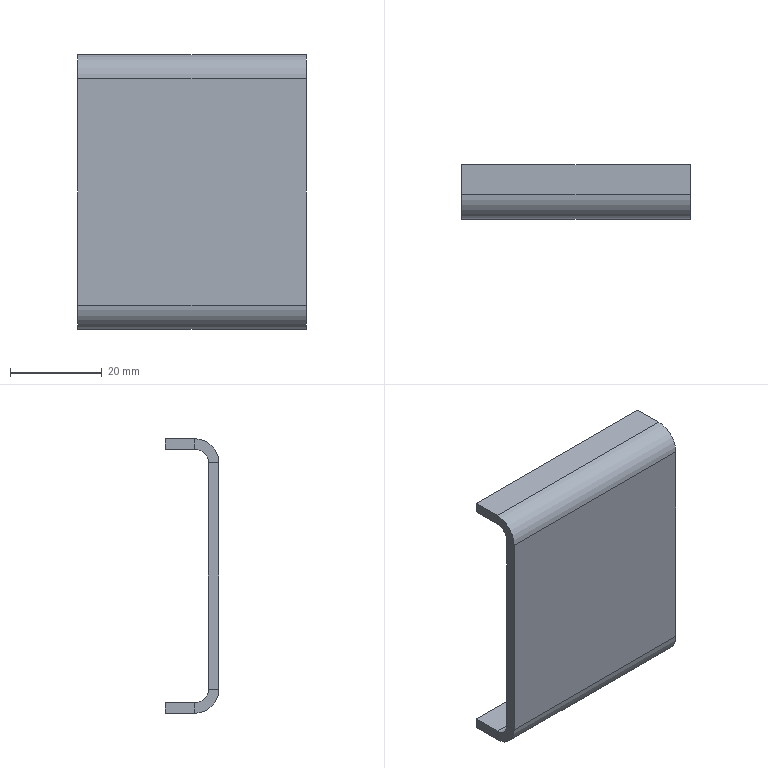Part | SolidWorks | features FlatPattern 1, SMBaseFlange 1, SheetMetal 1 | 1 solid | 22 faces | box 50 x 11.8 x 60 mm | volume 8675 mm3 | plane 18 | cylinder 4 | commonest cylinder face diameters 6 x2 10.6 x2
STEP:
#1=CARTESIAN_POINT('',(50.,-6.5,0.));
#2=VERTEX_POINT('',#1);
#3=CARTESIAN_POINT('',(50.,-6.5,-2.3));
#4=VERTEX_POINT('',#3);
#5=CARTESIAN_POINT('',(50.,-6.5,0.));
#6=DIRECTION('',(0.,0.,-1.));
#7=VECTOR('',#6,1000.);
#8=LINE('',#5,#7);
#9=EDGE_CURVE('',#2,#4,#8,.T.);
#10=ORIENTED_EDGE('',*,*,#9,.F.);
#11=CARTESIAN_POINT('',(50.,-11.8,-5.3));
#12=VERTEX_POINT('',#11);
#13=CARTESIAN_POINT('',(50.,-6.5,-5.3));
#14=DIRECTION('',(1.,0.,0.));
#15=DIRECTION('',(0.,0.,1.));
#16=AXIS2_PLACEMENT_3D('',#13,#14,#15);
#17=CIRCLE('',#16,5.3);
#18=EDGE_CURVE('',#2,#12,#17,.T.);
#19=ORIENTED_EDGE('',*,*,#18,.T.);
#20=CARTESIAN_POINT('',(50.,-9.5,-5.3));
#21=VERTEX_POINT('',#20);
#22=CARTESIAN_POINT('',(50.,-9.5,-5.3));
#23=DIRECTION('',(0.,-1.,0.));
#24=VECTOR('',#23,1000.);
#25=LINE('',#22,#24);
#26=EDGE_CURVE('',#21,#12,#25,.T.);
#27=ORIENTED_EDGE('',*,*,#26,.F.);
#28=CARTESIAN_POINT('',(50.,-6.5,-5.3));
#29=DIRECTION('',(1.,0.,0.));
#30=DIRECTION('',(0.,0.,-1.));
#31=AXIS2_PLACEMENT_3D('',#28,#29,#30);
#32=CIRCLE('',#31,3.);
#33=EDGE_CURVE('',#4,#21,#32,.T.);
#34=ORIENTED_EDGE('',*,*,#33,.F.);
#35=EDGE_LOOP('',(#10,#19,#27,#34));
#36=FACE_OUTER_BOUND('',#35,.T.);
#37=CARTESIAN_POINT('',(50.,-6.5,0.));
#38=DIRECTION('',(1.,0.,0.));
#39=DIRECTION('',(0.,0.,-1.));
#40=AXIS2_PLACEMENT_3D('',#37,#38,#39);
#41=PLANE('',#40);
#42=ADVANCED_FACE('',(#36),#41,.T.);
#43=CARTESIAN_POINT('',(50.,0.,0.));
#44=VERTEX_POINT('',#43);
#45=CARTESIAN_POINT('',(50.,0.,0.));
#46=DIRECTION('',(0.,-1.,0.));
#47=VECTOR('',#46,1000.);
#48=LINE('',#45,#47);
#49=EDGE_CURVE('',#44,#2,#48,.T.);
#50=ORIENTED_EDGE('',*,*,#49,.T.);
#51=ORIENTED_EDGE('',*,*,#9,.T.);
#52=CARTESIAN_POINT('',(50.,0.,-2.3));
#53=VERTEX_POINT('',#52);
#54=CARTESIAN_POINT('',(50.,0.,-2.3));
#55=DIRECTION('',(0.,-1.,0.));
#56=VECTOR('',#55,1000.);
#57=LINE('',#54,#56);
#58=EDGE_CURVE('',#53,#4,#57,.T.);
#59=ORIENTED_EDGE('',*,*,#58,.F.);
#60=CARTESIAN_POINT('',(50.,0.,0.));
#61=DIRECTION('',(0.,0.,-1.));
#62=VECTOR('',#61,1000.);
#63=LINE('',#60,#62);
#64=EDGE_CURVE('',#44,#53,#63,.T.);
#65=ORIENTED_EDGE('',*,*,#64,.F.);
#66=EDGE_LOOP('',(#50,#51,#59,#65));
#67=FACE_OUTER_BOUND('',#66,.T.);
#68=CARTESIAN_POINT('',(50.,-9.5,-5.3));
#69=DIRECTION('',(1.,0.,0.));
#70=DIRECTION('',(0.,0.,-1.));
#71=AXIS2_PLACEMENT_3D('',#68,#69,#70);
#72=PLANE('',#71);
#73=ADVANCED_FACE('',(#67),#72,.T.);
#74=CARTESIAN_POINT('',(0.,-11.8,-5.3));
#75=VERTEX_POINT('',#74);
#76=CARTESIAN_POINT('',(0.,-9.5,-5.3));
#77=VERTEX_POINT('',#76);
#78=CARTESIAN_POINT('',(0.,-11.8,-5.3));
#79=DIRECTION('',(0.,1.,0.));
#80=VECTOR('',#79,1000.);
#81=LINE('',#78,#80);
#82=EDGE_CURVE('',#75,#77,#81,.T.);
#83=ORIENTED_EDGE('',*,*,#82,.F.);
#84=CARTESIAN_POINT('',(0.,-6.5,0.));
#85=VERTEX_POINT('',#84);
#86=CARTESIAN_POINT('',(0.,-6.5,-5.3));
#87=DIRECTION('',(1.,0.,0.));
#88=DIRECTION('',(0.,0.,1.));
#89=AXIS2_PLACEMENT_3D('',#86,#87,#88);
#90=CIRCLE('',#89,5.3);
#91=EDGE_CURVE('',#85,#75,#90,.T.);
#92=ORIENTED_EDGE('',*,*,#91,.F.);
#93=CARTESIAN_POINT('',(0.,-6.5,-2.3));
#94=VERTEX_POINT('',#93);
#95=CARTESIAN_POINT('',(0.,-6.5,-2.3));
#96=DIRECTION('',(0.,0.,1.));
#97=VECTOR('',#96,1000.);
#98=LINE('',#95,#97);
#99=EDGE_CURVE('',#94,#85,#98,.T.);
#100=ORIENTED_EDGE('',*,*,#99,.F.);
#101=CARTESIAN_POINT('',(0.,-6.5,-5.3));
#102=DIRECTION('',(1.,0.,0.));
#103=DIRECTION('',(0.,0.,-1.));
#104=AXIS2_PLACEMENT_3D('',#101,#102,#103);
#105=CIRCLE('',#104,3.);
#106=EDGE_CURVE('',#94,#77,#105,.T.);
#107=ORIENTED_EDGE('',*,*,#106,.T.);
#108=EDGE_LOOP('',(#83,#92,#100,#107));
#109=FACE_OUTER_BOUND('',#108,.T.);
#110=CARTESIAN_POINT('',(0.,-11.8,-5.3));
#111=DIRECTION('',(-1.,0.,0.));
#112=DIRECTION('',(0.,0.,1.));
#113=AXIS2_PLACEMENT_3D('',#110,#111,#112);
#114=PLANE('',#113);
#115=ADVANCED_FACE('',(#109),#114,.T.);
#116=CARTESIAN_POINT('',(0.,-11.8,-54.7));
#117=VERTEX_POINT('',#116);
#118=CARTESIAN_POINT('',(0.,-11.8,0.));
#119=DIRECTION('',(0.,0.,-1.));
#120=VECTOR('',#119,1000.);
#121=LINE('',#118,#120);
#122=EDGE_CURVE('',#75,#117,#121,.T.);
#123=ORIENTED_EDGE('',*,*,#122,.F.);
#124=ORIENTED_EDGE('',*,*,#82,.T.);
#125=CARTESIAN_POINT('',(0.,-9.5,-54.7));
#126=VERTEX_POINT('',#125);
#127=CARTESIAN_POINT('',(0.,-9.5,0.));
#128=DIRECTION('',(0.,0.,-1.));
#129=VECTOR('',#128,1000.);
#130=LINE('',#127,#129);
#131=EDGE_CURVE('',#77,#126,#130,.T.);
#132=ORIENTED_EDGE('',*,*,#131,.T.);
#133=CARTESIAN_POINT('',(0.,-9.5,-54.7));
#134=DIRECTION('',(0.,-1.,0.));
#135=VECTOR('',#134,1000.);
#136=LINE('',#133,#135);
#137=EDGE_CURVE('',#126,#117,#136,.T.);
#138=ORIENTED_EDGE('',*,*,#137,.T.);
#139=EDGE_LOOP('',(#123,#124,#132,#138));
#140=FACE_OUTER_BOUND('',#139,.T.);
#141=CARTESIAN_POINT('',(0.,-6.5,-2.3));
#142=DIRECTION('',(-1.,0.,0.));
#143=DIRECTION('',(0.,0.,1.));
#144=AXIS2_PLACEMENT_3D('',#141,#142,#143);
#145=PLANE('',#144);
#146=ADVANCED_FACE('',(#140),#145,.T.);
#147=CARTESIAN_POINT('',(50.,-11.8,-54.7));
#148=VERTEX_POINT('',#147);
#149=CARTESIAN_POINT('',(50.,-9.5,-54.7));
#150=VERTEX_POINT('',#149);
#151=CARTESIAN_POINT('',(50.,-11.8,-54.7));
#152=DIRECTION('',(0.,1.,0.));
#153=VECTOR('',#152,1000.);
#154=LINE('',#151,#153);
#155=EDGE_CURVE('',#148,#150,#154,.T.);
#156=ORIENTED_EDGE('',*,*,#155,.F.);
#157=CARTESIAN_POINT('',(50.,-6.5,-60.));
#158=VERTEX_POINT('',#157);
#159=CARTESIAN_POINT('',(50.,-6.5,-54.7));
#160=DIRECTION('',(1.,0.,0.));
#161=DIRECTION('',(0.,0.,1.));
#162=AXIS2_PLACEMENT_3D('',#159,#160,#161);
#163=CIRCLE('',#162,5.3);
#164=EDGE_CURVE('',#148,#158,#163,.T.);
#165=ORIENTED_EDGE('',*,*,#164,.T.);
#166=CARTESIAN_POINT('',(50.,-6.5,-57.7));
#167=VERTEX_POINT('',#166);
#168=CARTESIAN_POINT('',(50.,-6.5,-57.7));
#169=DIRECTION('',(0.,0.,-1.));
#170=VECTOR('',#169,1000.);
#171=LINE('',#168,#170);
#172=EDGE_CURVE('',#167,#158,#171,.T.);
#173=ORIENTED_EDGE('',*,*,#172,.F.);
#174=CARTESIAN_POINT('',(50.,-6.5,-54.7));
#175=DIRECTION('',(1.,0.,0.));
#176=DIRECTION('',(0.,0.,-1.));
#177=AXIS2_PLACEMENT_3D('',#174,#175,#176);
#178=CIRCLE('',#177,3.);
#179=EDGE_CURVE('',#150,#167,#178,.T.);
#180=ORIENTED_EDGE('',*,*,#179,.F.);
#181=EDGE_LOOP('',(#156,#165,#173,#180));
#182=FACE_OUTER_BOUND('',#181,.T.);
#183=CARTESIAN_POINT('',(50.,-11.8,-54.7));
#184=DIRECTION('',(1.,0.,0.));
#185=DIRECTION('',(0.,0.,-1.));
#186=AXIS2_PLACEMENT_3D('',#183,#184,#185);
#187=PLANE('',#186);
#188=ADVANCED_FACE('',(#182),#187,.T.);
#189=CARTESIAN_POINT('',(50.,-11.8,0.));
#190=DIRECTION('',(0.,0.,-1.));
#191=VECTOR('',#190,1000.);
#192=LINE('',#189,#191);
#193=EDGE_CURVE('',#12,#148,#192,.T.);
#194=ORIENTED_EDGE('',*,*,#193,.T.);
#195=ORIENTED_EDGE('',*,*,#155,.T.);
#196=CARTESIAN_POINT('',(50.,-9.5,0.));
#197=DIRECTION('',(0.,0.,-1.));
#198=VECTOR('',#197,1000.);
#199=LINE('',#196,#198);
#200=EDGE_CURVE('',#21,#150,#199,.T.);
#201=ORIENTED_EDGE('',*,*,#200,.F.);
#202=ORIENTED_EDGE('',*,*,#26,.T.);
#203=EDGE_LOOP('',(#194,#195,#201,#202));
#204=FACE_OUTER_BOUND('',#203,.T.);
#205=CARTESIAN_POINT('',(50.,-6.5,-57.7));
#206=DIRECTION('',(1.,0.,0.));
#207=DIRECTION('',(0.,0.,-1.));
#208=AXIS2_PLACEMENT_3D('',#205,#206,#207);
#209=PLANE('',#208);
#210=ADVANCED_FACE('',(#204),#209,.T.);
#211=CARTESIAN_POINT('',(0.,-6.5,-60.));
#212=VERTEX_POINT('',#211);
#213=CARTESIAN_POINT('',(0.,-6.5,-57.7));
#214=VERTEX_POINT('',#213);
#215=CARTESIAN_POINT('',(0.,-6.5,-60.));
#216=DIRECTION('',(0.,0.,1.));
#217=VECTOR('',#216,1000.);
#218=LINE('',#215,#217);
#219=EDGE_CURVE('',#212,#214,#218,.T.);
#220=ORIENTED_EDGE('',*,*,#219,.F.);
#221=CARTESIAN_POINT('',(0.,-6.5,-54.7));
#222=DIRECTION('',(1.,0.,0.));
#223=DIRECTION('',(0.,0.,1.));
#224=AXIS2_PLACEMENT_3D('',#221,#222,#223);
#225=CIRCLE('',#224,5.3);
#226=EDGE_CURVE('',#117,#212,#225,.T.);
#227=ORIENTED_EDGE('',*,*,#226,.F.);
#228=ORIENTED_EDGE('',*,*,#137,.F.);
#229=CARTESIAN_POINT('',(0.,-6.5,-54.7));
#230=DIRECTION('',(1.,0.,0.));
#231=DIRECTION('',(0.,0.,-1.));
#232=AXIS2_PLACEMENT_3D('',#229,#230,#231);
#233=CIRCLE('',#232,3.);
#234=EDGE_CURVE('',#126,#214,#233,.T.);
#235=ORIENTED_EDGE('',*,*,#234,.T.);
#236=EDGE_LOOP('',(#220,#227,#228,#235));
#237=FACE_OUTER_BOUND('',#236,.T.);
#238=CARTESIAN_POINT('',(0.,-6.5,-60.));
#239=DIRECTION('',(-1.,0.,0.));
#240=DIRECTION('',(0.,0.,1.));
#241=AXIS2_PLACEMENT_3D('',#238,#239,#240);
#242=PLANE('',#241);
#243=ADVANCED_FACE('',(#237),#242,.T.);
#244=CARTESIAN_POINT('',(0.,0.,-60.));
#245=VERTEX_POINT('',#244);
#246=CARTESIAN_POINT('',(0.,-11.8,-60.));
#247=DIRECTION('',(0.,1.,0.));
#248=VECTOR('',#247,1000.);
#249=LINE('',#246,#248);
#250=EDGE_CURVE('',#212,#245,#249,.T.);
#251=ORIENTED_EDGE('',*,*,#250,.F.);
#252=ORIENTED_EDGE('',*,*,#219,.T.);
#253=CARTESIAN_POINT('',(0.,0.,-57.7));
#254=VERTEX_POINT('',#253);
#255=CARTESIAN_POINT('',(0.,-11.8,-57.7));
#256=DIRECTION('',(0.,1.,0.));
#257=VECTOR('',#256,1000.);
#258=LINE('',#255,#257);
#259=EDGE_CURVE('',#214,#254,#258,.T.);
#260=ORIENTED_EDGE('',*,*,#259,.T.);
#261=CARTESIAN_POINT('',(0.,0.,-57.7));
#262=DIRECTION('',(0.,0.,-1.));
#263=VECTOR('',#262,1000.);
#264=LINE('',#261,#263);
#265=EDGE_CURVE('',#254,#245,#264,.T.);
#266=ORIENTED_EDGE('',*,*,#265,.T.);
#267=EDGE_LOOP('',(#251,#252,#260,#266));
#268=FACE_OUTER_BOUND('',#267,.T.);
#269=CARTESIAN_POINT('',(0.,-9.5,-54.7));
#270=DIRECTION('',(-1.,0.,0.));
#271=DIRECTION('',(0.,0.,1.));
#272=AXIS2_PLACEMENT_3D('',#269,#270,#271);
#273=PLANE('',#272);
#274=ADVANCED_FACE('',(#268),#273,.T.);
#275=ORIENTED_EDGE('',*,*,#250,.T.);
#276=CARTESIAN_POINT('',(50.,0.,-60.));
#277=VERTEX_POINT('',#276);
#278=CARTESIAN_POINT('',(50.,0.,-60.));
#279=DIRECTION('',(-1.,0.,0.));
#280=VECTOR('',#279,1000.);
#281=LINE('',#278,#280);
#282=EDGE_CURVE('',#277,#245,#281,.T.);
#283=ORIENTED_EDGE('',*,*,#282,.F.);
#284=CARTESIAN_POINT('',(50.,-11.8,-60.));
#285=DIRECTION('',(0.,1.,0.));
#286=VECTOR('',#285,1000.);
#287=LINE('',#284,#286);
#288=EDGE_CURVE('',#158,#277,#287,.T.);
#289=ORIENTED_EDGE('',*,*,#288,.F.);
#290=CARTESIAN_POINT('',(50.,-6.5,-60.));
#291=DIRECTION('',(-1.,0.,0.));
#292=VECTOR('',#291,1000.);
#293=LINE('',#290,#292);
#294=EDGE_CURVE('',#158,#212,#293,.T.);
#295=ORIENTED_EDGE('',*,*,#294,.T.);
#296=EDGE_LOOP('',(#275,#283,#289,#295));
#297=FACE_OUTER_BOUND('',#296,.T.);
#298=CARTESIAN_POINT('',(50.,-11.8,-60.));
#299=DIRECTION('',(0.,0.,1.));
#300=DIRECTION('',(1.,0.,0.));
#301=AXIS2_PLACEMENT_3D('',#298,#299,#300);
#302=PLANE('',#301);
#303=ADVANCED_FACE('',(#297),#302,.F.);
#304=ORIENTED_EDGE('',*,*,#265,.F.);
#305=CARTESIAN_POINT('',(50.,0.,-57.7));
#306=VERTEX_POINT('',#305);
#307=CARTESIAN_POINT('',(50.,0.,-57.7));
#308=DIRECTION('',(-1.,0.,0.));
#309=VECTOR('',#308,1000.);
#310=LINE('',#307,#309);
#311=EDGE_CURVE('',#306,#254,#310,.T.);
#312=ORIENTED_EDGE('',*,*,#311,.F.);
#313=CARTESIAN_POINT('',(50.,0.,-57.7));
#314=DIRECTION('',(0.,0.,-1.));
#315=VECTOR('',#314,1000.);
#316=LINE('',#313,#315);
#317=EDGE_CURVE('',#306,#277,#316,.T.);
#318=ORIENTED_EDGE('',*,*,#317,.T.);
#319=ORIENTED_EDGE('',*,*,#282,.T.);
#320=EDGE_LOOP('',(#304,#312,#318,#319));
#321=FACE_OUTER_BOUND('',#320,.T.);
#322=CARTESIAN_POINT('',(50.,0.,-57.7));
#323=DIRECTION('',(0.,1.,0.));
#324=DIRECTION('',(0.,0.,1.));
#325=AXIS2_PLACEMENT_3D('',#322,#323,#324);
#326=PLANE('',#325);
#327=ADVANCED_FACE('',(#321),#326,.T.);
#328=ORIENTED_EDGE('',*,*,#259,.F.);
#329=CARTESIAN_POINT('',(50.,-6.5,-57.7));
#330=DIRECTION('',(-1.,0.,0.));
#331=VECTOR('',#330,1000.);
#332=LINE('',#329,#331);
#333=EDGE_CURVE('',#167,#214,#332,.T.);
#334=ORIENTED_EDGE('',*,*,#333,.F.);
#335=CARTESIAN_POINT('',(50.,-11.8,-57.7));
#336=DIRECTION('',(0.,1.,0.));
#337=VECTOR('',#336,1000.);
#338=LINE('',#335,#337);
#339=EDGE_CURVE('',#167,#306,#338,.T.);
#340=ORIENTED_EDGE('',*,*,#339,.T.);
#341=ORIENTED_EDGE('',*,*,#311,.T.);
#342=EDGE_LOOP('',(#328,#334,#340,#341));
#343=FACE_OUTER_BOUND('',#342,.T.);
#344=CARTESIAN_POINT('',(50.,-11.8,-57.7));
#345=DIRECTION('',(0.,0.,1.));
#346=DIRECTION('',(1.,0.,0.));
#347=AXIS2_PLACEMENT_3D('',#344,#345,#346);
#348=PLANE('',#347);
#349=ADVANCED_FACE('',(#343),#348,.T.);
#350=ORIENTED_EDGE('',*,*,#234,.F.);
#351=CARTESIAN_POINT('',(50.,-9.5,-54.7));
#352=DIRECTION('',(-1.,0.,0.));
#353=VECTOR('',#352,1000.);
#354=LINE('',#351,#353);
#355=EDGE_CURVE('',#150,#126,#354,.T.);
#356=ORIENTED_EDGE('',*,*,#355,.F.);
#357=ORIENTED_EDGE('',*,*,#179,.T.);
#358=ORIENTED_EDGE('',*,*,#333,.T.);
#359=EDGE_LOOP('',(#350,#356,#357,#358));
#360=FACE_OUTER_BOUND('',#359,.T.);
#361=CARTESIAN_POINT('',(50.,-6.5,-54.7));
#362=DIRECTION('',(-1.,0.,0.));
#363=DIRECTION('',(0.,0.,1.));
#364=AXIS2_PLACEMENT_3D('',#361,#362,#363);
#365=CYLINDRICAL_SURFACE('',#364,3.);
#366=ADVANCED_FACE('',(#360),#365,.F.);
#367=ORIENTED_EDGE('',*,*,#131,.F.);
#368=CARTESIAN_POINT('',(50.,-9.5,-5.3));
#369=DIRECTION('',(-1.,0.,0.));
#370=VECTOR('',#369,1000.);
#371=LINE('',#368,#370);
#372=EDGE_CURVE('',#21,#77,#371,.T.);
#373=ORIENTED_EDGE('',*,*,#372,.F.);
#374=ORIENTED_EDGE('',*,*,#200,.T.);
#375=ORIENTED_EDGE('',*,*,#355,.T.);
#376=EDGE_LOOP('',(#367,#373,#374,#375));
#377=FACE_OUTER_BOUND('',#376,.T.);
#378=CARTESIAN_POINT('',(50.,-9.5,0.));
#379=DIRECTION('',(0.,1.,0.));
#380=DIRECTION('',(0.,0.,1.));
#381=AXIS2_PLACEMENT_3D('',#378,#379,#380);
#382=PLANE('',#381);
#383=ADVANCED_FACE('',(#377),#382,.T.);
#384=ORIENTED_EDGE('',*,*,#106,.F.);
#385=CARTESIAN_POINT('',(50.,-6.5,-2.3));
#386=DIRECTION('',(-1.,0.,0.));
#387=VECTOR('',#386,1000.);
#388=LINE('',#385,#387);
#389=EDGE_CURVE('',#4,#94,#388,.T.);
#390=ORIENTED_EDGE('',*,*,#389,.F.);
#391=ORIENTED_EDGE('',*,*,#33,.T.);
#392=ORIENTED_EDGE('',*,*,#372,.T.);
#393=EDGE_LOOP('',(#384,#390,#391,#392));
#394=FACE_OUTER_BOUND('',#393,.T.);
#395=CARTESIAN_POINT('',(50.,-6.5,-5.3));
#396=DIRECTION('',(-1.,0.,0.));
#397=DIRECTION('',(0.,0.,1.));
#398=AXIS2_PLACEMENT_3D('',#395,#396,#397);
#399=CYLINDRICAL_SURFACE('',#398,3.);
#400=ADVANCED_FACE('',(#394),#399,.F.);
#401=CARTESIAN_POINT('',(0.,0.,-2.3));
#402=VERTEX_POINT('',#401);
#403=CARTESIAN_POINT('',(0.,0.,-2.3));
#404=DIRECTION('',(0.,-1.,0.));
#405=VECTOR('',#404,1000.);
#406=LINE('',#403,#405);
#407=EDGE_CURVE('',#402,#94,#406,.T.);
#408=ORIENTED_EDGE('',*,*,#407,.F.);
#409=CARTESIAN_POINT('',(50.,0.,-2.3));
#410=DIRECTION('',(-1.,0.,0.));
#411=VECTOR('',#410,1000.);
#412=LINE('',#409,#411);
#413=EDGE_CURVE('',#53,#402,#412,.T.);
#414=ORIENTED_EDGE('',*,*,#413,.F.);
#415=ORIENTED_EDGE('',*,*,#58,.T.);
#416=ORIENTED_EDGE('',*,*,#389,.T.);
#417=EDGE_LOOP('',(#408,#414,#415,#416));
#418=FACE_OUTER_BOUND('',#417,.T.);
#419=CARTESIAN_POINT('',(50.,0.,-2.3));
#420=DIRECTION('',(0.,0.,-1.));
#421=DIRECTION('',(0.,1.,0.));
#422=AXIS2_PLACEMENT_3D('',#419,#420,#421);
#423=PLANE('',#422);
#424=ADVANCED_FACE('',(#418),#423,.T.);
#425=CARTESIAN_POINT('',(0.,0.,0.));
#426=VERTEX_POINT('',#425);
#427=CARTESIAN_POINT('',(0.,0.,0.));
#428=DIRECTION('',(0.,0.,-1.));
#429=VECTOR('',#428,1000.);
#430=LINE('',#427,#429);
#431=EDGE_CURVE('',#426,#402,#430,.T.);
#432=ORIENTED_EDGE('',*,*,#431,.F.);
#433=CARTESIAN_POINT('',(50.,0.,0.));
#434=DIRECTION('',(-1.,0.,0.));
#435=VECTOR('',#434,1000.);
#436=LINE('',#433,#435);
#437=EDGE_CURVE('',#44,#426,#436,.T.);
#438=ORIENTED_EDGE('',*,*,#437,.F.);
#439=ORIENTED_EDGE('',*,*,#64,.T.);
#440=ORIENTED_EDGE('',*,*,#413,.T.);
#441=EDGE_LOOP('',(#432,#438,#439,#440));
#442=FACE_OUTER_BOUND('',#441,.T.);
#443=CARTESIAN_POINT('',(50.,0.,0.));
#444=DIRECTION('',(0.,1.,0.));
#445=DIRECTION('',(0.,0.,1.));
#446=AXIS2_PLACEMENT_3D('',#443,#444,#445);
#447=PLANE('',#446);
#448=ADVANCED_FACE('',(#442),#447,.T.);
#449=CARTESIAN_POINT('',(0.,0.,0.));
#450=DIRECTION('',(0.,-1.,0.));
#451=VECTOR('',#450,1000.);
#452=LINE('',#449,#451);
#453=EDGE_CURVE('',#426,#85,#452,.T.);
#454=ORIENTED_EDGE('',*,*,#453,.T.);
#455=CARTESIAN_POINT('',(50.,-6.5,0.));
#456=DIRECTION('',(-1.,0.,0.));
#457=VECTOR('',#456,1000.);
#458=LINE('',#455,#457);
#459=EDGE_CURVE('',#2,#85,#458,.T.);
#460=ORIENTED_EDGE('',*,*,#459,.F.);
#461=ORIENTED_EDGE('',*,*,#49,.F.);
#462=ORIENTED_EDGE('',*,*,#437,.T.);
#463=EDGE_LOOP('',(#454,#460,#461,#462));
#464=FACE_OUTER_BOUND('',#463,.T.);
#465=CARTESIAN_POINT('',(50.,0.,0.));
#466=DIRECTION('',(0.,0.,-1.));
#467=DIRECTION('',(0.,1.,0.));
#468=AXIS2_PLACEMENT_3D('',#465,#466,#467);
#469=PLANE('',#468);
#470=ADVANCED_FACE('',(#464),#469,.F.);
#471=ORIENTED_EDGE('',*,*,#91,.T.);
#472=CARTESIAN_POINT('',(50.,-11.8,-5.3));
#473=DIRECTION('',(-1.,0.,0.));
#474=VECTOR('',#473,1000.);
#475=LINE('',#472,#474);
#476=EDGE_CURVE('',#12,#75,#475,.T.);
#477=ORIENTED_EDGE('',*,*,#476,.F.);
#478=ORIENTED_EDGE('',*,*,#18,.F.);
#479=ORIENTED_EDGE('',*,*,#459,.T.);
#480=EDGE_LOOP('',(#471,#477,#478,#479));
#481=FACE_OUTER_BOUND('',#480,.T.);
#482=CARTESIAN_POINT('',(50.,-6.5,-5.3));
#483=DIRECTION('',(-1.,0.,0.));
#484=DIRECTION('',(0.,0.,1.));
#485=AXIS2_PLACEMENT_3D('',#482,#483,#484);
#486=CYLINDRICAL_SURFACE('',#485,5.3);
#487=ADVANCED_FACE('',(#481),#486,.T.);
#488=ORIENTED_EDGE('',*,*,#122,.T.);
#489=CARTESIAN_POINT('',(50.,-11.8,-54.7));
#490=DIRECTION('',(-1.,0.,0.));
#491=VECTOR('',#490,1000.);
#492=LINE('',#489,#491);
#493=EDGE_CURVE('',#148,#117,#492,.T.);
#494=ORIENTED_EDGE('',*,*,#493,.F.);
#495=ORIENTED_EDGE('',*,*,#193,.F.);
#496=ORIENTED_EDGE('',*,*,#476,.T.);
#497=EDGE_LOOP('',(#488,#494,#495,#496));
#498=FACE_OUTER_BOUND('',#497,.T.);
#499=CARTESIAN_POINT('',(50.,-11.8,0.));
#500=DIRECTION('',(0.,1.,0.));
#501=DIRECTION('',(0.,0.,1.));
#502=AXIS2_PLACEMENT_3D('',#499,#500,#501);
#503=PLANE('',#502);
#504=ADVANCED_FACE('',(#498),#503,.F.);
#505=ORIENTED_EDGE('',*,*,#226,.T.);
#506=ORIENTED_EDGE('',*,*,#294,.F.);
#507=ORIENTED_EDGE('',*,*,#164,.F.);
#508=ORIENTED_EDGE('',*,*,#493,.T.);
#509=EDGE_LOOP('',(#505,#506,#507,#508));
#510=FACE_OUTER_BOUND('',#509,.T.);
#511=CARTESIAN_POINT('',(50.,-6.5,-54.7));
#512=DIRECTION('',(-1.,0.,0.));
#513=DIRECTION('',(0.,0.,1.));
#514=AXIS2_PLACEMENT_3D('',#511,#512,#513);
#515=CYLINDRICAL_SURFACE('',#514,5.3);
#516=ADVANCED_FACE('',(#510),#515,.T.);
#517=ORIENTED_EDGE('',*,*,#288,.T.);
#518=ORIENTED_EDGE('',*,*,#317,.F.);
#519=ORIENTED_EDGE('',*,*,#339,.F.);
#520=ORIENTED_EDGE('',*,*,#172,.T.);
#521=EDGE_LOOP('',(#517,#518,#519,#520));
#522=FACE_OUTER_BOUND('',#521,.T.);
#523=CARTESIAN_POINT('',(50.,-6.5,-54.7));
#524=DIRECTION('',(1.,0.,0.));
#525=DIRECTION('',(0.,0.,-1.));
#526=AXIS2_PLACEMENT_3D('',#523,#524,#525);
#527=PLANE('',#526);
#528=ADVANCED_FACE('',(#522),#527,.T.);
#529=ORIENTED_EDGE('',*,*,#407,.T.);
#530=ORIENTED_EDGE('',*,*,#99,.T.);
#531=ORIENTED_EDGE('',*,*,#453,.F.);
#532=ORIENTED_EDGE('',*,*,#431,.T.);
#533=EDGE_LOOP('',(#529,#530,#531,#532));
#534=FACE_OUTER_BOUND('',#533,.T.);
#535=CARTESIAN_POINT('',(0.,-6.5,-54.7));
#536=DIRECTION('',(1.,0.,0.));
#537=DIRECTION('',(0.,0.,-1.));
#538=AXIS2_PLACEMENT_3D('',#535,#536,#537);
#539=PLANE('',#538);
#540=ADVANCED_FACE('',(#534),#539,.F.);
#541=CLOSED_SHELL('',(#42,#73,#115,#146,#188,#210,#243,#274,#303,#327,#349,#366,#383,#400,#424,#448,#470,#487,#504,#516,#528,#540));
#542=MANIFOLD_SOLID_BREP('',#541);
#543=CARTESIAN_POINT('',(0.,0.,0.));
#544=DIRECTION('',(0.,0.,1.));
#545=DIRECTION('',(1.,0.,0.));
#546=AXIS2_PLACEMENT_3D('',#543,#544,#545);
#547=(LENGTH_UNIT()NAMED_UNIT(*)SI_UNIT(.MILLI.,.METRE.));
#548=UNCERTAINTY_MEASURE_WITH_UNIT(LENGTH_MEASURE(0.00001),#547,'','');
#549=(NAMED_UNIT(*)PLANE_ANGLE_UNIT()SI_UNIT($,.RADIAN.));
#550=(NAMED_UNIT(*)SI_UNIT($,.STERADIAN.)SOLID_ANGLE_UNIT());
#551=(GEOMETRIC_REPRESENTATION_CONTEXT(3)GLOBAL_UNCERTAINTY_ASSIGNED_CONTEXT((#548))GLOBAL_UNIT_ASSIGNED_CONTEXT((#547,#549,#550))REPRESENTATION_CONTEXT('',''));
#552=ADVANCED_BREP_SHAPE_REPRESENTATION('',(#542,#546),#551);